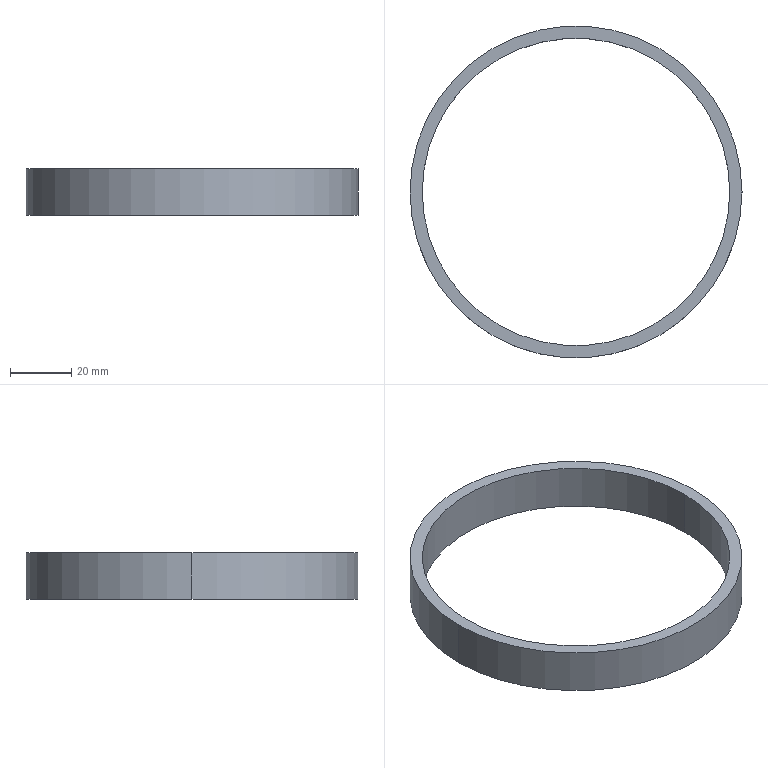Part | SolidWorks | features Extrusion 1 | 1 solid | 6 faces | box 108 x 108 x 15 mm | volume 19604 mm3 | cylinder 4 | plane 2 | commonest cylinder face diameters 100 x2 108 x2
STEP:
#1=CARTESIAN_POINT('',(-50.,0.,15.));
#2=VERTEX_POINT('',#1);
#3=CARTESIAN_POINT('',(50.,0.,15.));
#4=VERTEX_POINT('',#3);
#5=CARTESIAN_POINT('',(0.,0.,15.));
#6=DIRECTION('',(0.,0.,1.));
#7=DIRECTION('',(1.,0.,0.));
#8=AXIS2_PLACEMENT_3D('',#5,#6,#7);
#9=CIRCLE('',#8,50.);
#10=EDGE_CURVE('',#2,#4,#9,.T.);
#11=ORIENTED_EDGE('',*,*,#10,.T.);
#12=CARTESIAN_POINT('',(50.,0.,0.));
#13=VERTEX_POINT('',#12);
#14=CARTESIAN_POINT('',(50.,0.,15.));
#15=DIRECTION('',(0.,0.,-1.));
#16=VECTOR('',#15,1000.);
#17=LINE('',#14,#16);
#18=EDGE_CURVE('',#4,#13,#17,.T.);
#19=ORIENTED_EDGE('',*,*,#18,.T.);
#20=CARTESIAN_POINT('',(-50.,0.,0.));
#21=VERTEX_POINT('',#20);
#22=CARTESIAN_POINT('',(0.,0.,0.));
#23=DIRECTION('',(0.,0.,1.));
#24=DIRECTION('',(1.,0.,0.));
#25=AXIS2_PLACEMENT_3D('',#22,#23,#24);
#26=CIRCLE('',#25,50.);
#27=EDGE_CURVE('',#21,#13,#26,.T.);
#28=ORIENTED_EDGE('',*,*,#27,.F.);
#29=CARTESIAN_POINT('',(-50.,0.,15.));
#30=DIRECTION('',(0.,0.,-1.));
#31=VECTOR('',#30,1000.);
#32=LINE('',#29,#31);
#33=EDGE_CURVE('',#2,#21,#32,.T.);
#34=ORIENTED_EDGE('',*,*,#33,.F.);
#35=EDGE_LOOP('',(#11,#19,#28,#34));
#36=FACE_OUTER_BOUND('',#35,.T.);
#37=CARTESIAN_POINT('',(0.,0.,15.));
#38=DIRECTION('',(0.,0.,-1.));
#39=DIRECTION('',(-1.,0.,0.));
#40=AXIS2_PLACEMENT_3D('',#37,#38,#39);
#41=CYLINDRICAL_SURFACE('',#40,50.);
#42=ADVANCED_FACE('',(#36),#41,.F.);
#43=CARTESIAN_POINT('',(54.,0.,15.));
#44=VERTEX_POINT('',#43);
#45=CARTESIAN_POINT('',(-54.,0.,15.));
#46=VERTEX_POINT('',#45);
#47=CARTESIAN_POINT('',(0.,0.,15.));
#48=DIRECTION('',(0.,0.,1.));
#49=DIRECTION('',(1.,0.,0.));
#50=AXIS2_PLACEMENT_3D('',#47,#48,#49);
#51=CIRCLE('',#50,54.);
#52=EDGE_CURVE('',#44,#46,#51,.T.);
#53=ORIENTED_EDGE('',*,*,#52,.F.);
#54=CARTESIAN_POINT('',(54.,0.,0.));
#55=VERTEX_POINT('',#54);
#56=CARTESIAN_POINT('',(54.,0.,15.));
#57=DIRECTION('',(0.,0.,-1.));
#58=VECTOR('',#57,1000.);
#59=LINE('',#56,#58);
#60=EDGE_CURVE('',#44,#55,#59,.T.);
#61=ORIENTED_EDGE('',*,*,#60,.T.);
#62=CARTESIAN_POINT('',(-54.,0.,0.));
#63=VERTEX_POINT('',#62);
#64=CARTESIAN_POINT('',(0.,0.,0.));
#65=DIRECTION('',(0.,0.,1.));
#66=DIRECTION('',(1.,0.,0.));
#67=AXIS2_PLACEMENT_3D('',#64,#65,#66);
#68=CIRCLE('',#67,54.);
#69=EDGE_CURVE('',#55,#63,#68,.T.);
#70=ORIENTED_EDGE('',*,*,#69,.T.);
#71=CARTESIAN_POINT('',(-54.,0.,15.));
#72=DIRECTION('',(0.,0.,-1.));
#73=VECTOR('',#72,1000.);
#74=LINE('',#71,#73);
#75=EDGE_CURVE('',#46,#63,#74,.T.);
#76=ORIENTED_EDGE('',*,*,#75,.F.);
#77=EDGE_LOOP('',(#53,#61,#70,#76));
#78=FACE_OUTER_BOUND('',#77,.T.);
#79=CARTESIAN_POINT('',(0.,0.,15.));
#80=DIRECTION('',(0.,0.,-1.));
#81=DIRECTION('',(-1.,0.,0.));
#82=AXIS2_PLACEMENT_3D('',#79,#80,#81);
#83=CYLINDRICAL_SURFACE('',#82,54.);
#84=ADVANCED_FACE('',(#78),#83,.T.);
#85=CARTESIAN_POINT('',(0.,0.,15.));
#86=DIRECTION('',(0.,0.,1.));
#87=DIRECTION('',(1.,0.,0.));
#88=AXIS2_PLACEMENT_3D('',#85,#86,#87);
#89=CIRCLE('',#88,54.);
#90=EDGE_CURVE('',#46,#44,#89,.T.);
#91=ORIENTED_EDGE('',*,*,#90,.T.);
#92=ORIENTED_EDGE('',*,*,#52,.T.);
#93=EDGE_LOOP('',(#91,#92));
#94=FACE_OUTER_BOUND('',#93,.T.);
#95=ORIENTED_EDGE('',*,*,#10,.F.);
#96=CARTESIAN_POINT('',(0.,0.,15.));
#97=DIRECTION('',(0.,0.,1.));
#98=DIRECTION('',(1.,0.,0.));
#99=AXIS2_PLACEMENT_3D('',#96,#97,#98);
#100=CIRCLE('',#99,50.);
#101=EDGE_CURVE('',#4,#2,#100,.T.);
#102=ORIENTED_EDGE('',*,*,#101,.F.);
#103=EDGE_LOOP('',(#95,#102));
#104=FACE_BOUND('',#103,.T.);
#105=CARTESIAN_POINT('',(0.,0.,15.));
#106=DIRECTION('',(0.,0.,1.));
#107=DIRECTION('',(1.,0.,0.));
#108=AXIS2_PLACEMENT_3D('',#105,#106,#107);
#109=PLANE('',#108);
#110=ADVANCED_FACE('',(#94,#104),#109,.T.);
#111=CARTESIAN_POINT('',(0.,0.,0.));
#112=DIRECTION('',(0.,0.,1.));
#113=DIRECTION('',(1.,0.,0.));
#114=AXIS2_PLACEMENT_3D('',#111,#112,#113);
#115=CIRCLE('',#114,54.);
#116=EDGE_CURVE('',#63,#55,#115,.T.);
#117=ORIENTED_EDGE('',*,*,#116,.F.);
#118=ORIENTED_EDGE('',*,*,#69,.F.);
#119=EDGE_LOOP('',(#117,#118));
#120=FACE_OUTER_BOUND('',#119,.T.);
#121=ORIENTED_EDGE('',*,*,#27,.T.);
#122=CARTESIAN_POINT('',(0.,0.,0.));
#123=DIRECTION('',(0.,0.,1.));
#124=DIRECTION('',(1.,0.,0.));
#125=AXIS2_PLACEMENT_3D('',#122,#123,#124);
#126=CIRCLE('',#125,50.);
#127=EDGE_CURVE('',#13,#21,#126,.T.);
#128=ORIENTED_EDGE('',*,*,#127,.T.);
#129=EDGE_LOOP('',(#121,#128));
#130=FACE_BOUND('',#129,.T.);
#131=CARTESIAN_POINT('',(0.,0.,0.));
#132=DIRECTION('',(0.,0.,1.));
#133=DIRECTION('',(1.,0.,0.));
#134=AXIS2_PLACEMENT_3D('',#131,#132,#133);
#135=PLANE('',#134);
#136=ADVANCED_FACE('',(#120,#130),#135,.F.);
#137=ORIENTED_EDGE('',*,*,#60,.F.);
#138=ORIENTED_EDGE('',*,*,#90,.F.);
#139=ORIENTED_EDGE('',*,*,#75,.T.);
#140=ORIENTED_EDGE('',*,*,#116,.T.);
#141=EDGE_LOOP('',(#137,#138,#139,#140));
#142=FACE_OUTER_BOUND('',#141,.T.);
#143=CARTESIAN_POINT('',(0.,0.,15.));
#144=DIRECTION('',(0.,0.,-1.));
#145=DIRECTION('',(-1.,0.,0.));
#146=AXIS2_PLACEMENT_3D('',#143,#144,#145);
#147=CYLINDRICAL_SURFACE('',#146,54.);
#148=ADVANCED_FACE('',(#142),#147,.T.);
#149=ORIENTED_EDGE('',*,*,#18,.F.);
#150=ORIENTED_EDGE('',*,*,#101,.T.);
#151=ORIENTED_EDGE('',*,*,#33,.T.);
#152=ORIENTED_EDGE('',*,*,#127,.F.);
#153=EDGE_LOOP('',(#149,#150,#151,#152));
#154=FACE_OUTER_BOUND('',#153,.T.);
#155=CARTESIAN_POINT('',(0.,0.,15.));
#156=DIRECTION('',(0.,0.,-1.));
#157=DIRECTION('',(-1.,0.,0.));
#158=AXIS2_PLACEMENT_3D('',#155,#156,#157);
#159=CYLINDRICAL_SURFACE('',#158,50.);
#160=ADVANCED_FACE('',(#154),#159,.F.);
#161=CLOSED_SHELL('',(#42,#84,#110,#136,#148,#160));
#162=MANIFOLD_SOLID_BREP('',#161);
#163=CARTESIAN_POINT('',(0.,0.,0.));
#164=DIRECTION('',(0.,0.,1.));
#165=DIRECTION('',(1.,0.,0.));
#166=AXIS2_PLACEMENT_3D('',#163,#164,#165);
#167=(LENGTH_UNIT()NAMED_UNIT(*)SI_UNIT(.MILLI.,.METRE.));
#168=UNCERTAINTY_MEASURE_WITH_UNIT(LENGTH_MEASURE(0.00001),#167,'','');
#169=(NAMED_UNIT(*)PLANE_ANGLE_UNIT()SI_UNIT($,.RADIAN.));
#170=(NAMED_UNIT(*)SI_UNIT($,.STERADIAN.)SOLID_ANGLE_UNIT());
#171=(GEOMETRIC_REPRESENTATION_CONTEXT(3)GLOBAL_UNCERTAINTY_ASSIGNED_CONTEXT((#168))GLOBAL_UNIT_ASSIGNED_CONTEXT((#167,#169,#170))REPRESENTATION_CONTEXT('',''));
#172=ADVANCED_BREP_SHAPE_REPRESENTATION('',(#162,#166),#171);